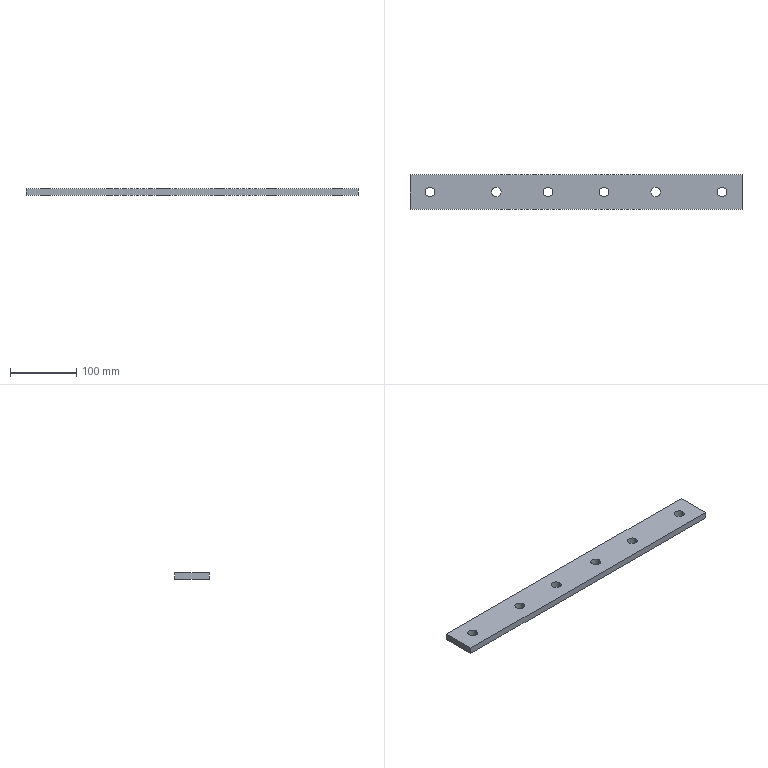Part | SolidWorks | features FlatPattern 1, ICE 1, MirrorPattern 1, SMBaseFlange 1, SheetMetal 1 | 1 solid | 18 faces | box 500 x 52 x 10 mm | volume 250092 mm3 | cylinder 12 | plane 6 | commonest cylinder face diameters 14.5 x12
STEP:
#1=CARTESIAN_POINT('',(-34.75,0.,-10.));
#2=VERTEX_POINT('',#1);
#3=CARTESIAN_POINT('',(-49.25,0.,-10.));
#4=VERTEX_POINT('',#3);
#5=CARTESIAN_POINT('',(-42.,0.,-10.));
#6=DIRECTION('',(0.,0.,-1.));
#7=DIRECTION('',(-1.,0.,0.));
#8=AXIS2_PLACEMENT_3D('',#5,#6,#7);
#9=CIRCLE('',#8,7.25);
#10=EDGE_CURVE('',#2,#4,#9,.T.);
#11=ORIENTED_EDGE('',*,*,#10,.T.);
#12=CARTESIAN_POINT('',(-49.25,0.,0.));
#13=VERTEX_POINT('',#12);
#14=CARTESIAN_POINT('',(-49.25,0.,-10.));
#15=DIRECTION('',(0.,0.,1.));
#16=VECTOR('',#15,1000.);
#17=LINE('',#14,#16);
#18=EDGE_CURVE('',#4,#13,#17,.T.);
#19=ORIENTED_EDGE('',*,*,#18,.T.);
#20=CARTESIAN_POINT('',(-34.75,0.,0.));
#21=VERTEX_POINT('',#20);
#22=CARTESIAN_POINT('',(-42.,0.,0.));
#23=DIRECTION('',(0.,0.,-1.));
#24=DIRECTION('',(1.,0.,0.));
#25=AXIS2_PLACEMENT_3D('',#22,#23,#24);
#26=CIRCLE('',#25,7.25);
#27=EDGE_CURVE('',#21,#13,#26,.T.);
#28=ORIENTED_EDGE('',*,*,#27,.F.);
#29=CARTESIAN_POINT('',(-34.75,0.,-10.));
#30=DIRECTION('',(0.,0.,1.));
#31=VECTOR('',#30,1000.);
#32=LINE('',#29,#31);
#33=EDGE_CURVE('',#2,#21,#32,.T.);
#34=ORIENTED_EDGE('',*,*,#33,.F.);
#35=EDGE_LOOP('',(#11,#19,#28,#34));
#36=FACE_OUTER_BOUND('',#35,.T.);
#37=CARTESIAN_POINT('',(-42.,0.,-10.));
#38=DIRECTION('',(0.,0.,1.));
#39=DIRECTION('',(1.,0.,0.));
#40=AXIS2_PLACEMENT_3D('',#37,#38,#39);
#41=CYLINDRICAL_SURFACE('',#40,7.25);
#42=ADVANCED_FACE('',(#36),#41,.F.);
#43=CARTESIAN_POINT('',(-112.75,0.,-10.));
#44=VERTEX_POINT('',#43);
#45=CARTESIAN_POINT('',(-127.25,0.,-10.));
#46=VERTEX_POINT('',#45);
#47=CARTESIAN_POINT('',(-120.,0.,-10.));
#48=DIRECTION('',(0.,0.,-1.));
#49=DIRECTION('',(-1.,0.,0.));
#50=AXIS2_PLACEMENT_3D('',#47,#48,#49);
#51=CIRCLE('',#50,7.25);
#52=EDGE_CURVE('',#44,#46,#51,.T.);
#53=ORIENTED_EDGE('',*,*,#52,.T.);
#54=CARTESIAN_POINT('',(-127.25,0.,0.));
#55=VERTEX_POINT('',#54);
#56=CARTESIAN_POINT('',(-127.25,0.,-10.));
#57=DIRECTION('',(0.,0.,1.));
#58=VECTOR('',#57,1000.);
#59=LINE('',#56,#58);
#60=EDGE_CURVE('',#46,#55,#59,.T.);
#61=ORIENTED_EDGE('',*,*,#60,.T.);
#62=CARTESIAN_POINT('',(-112.75,0.,0.));
#63=VERTEX_POINT('',#62);
#64=CARTESIAN_POINT('',(-120.,0.,0.));
#65=DIRECTION('',(0.,0.,-1.));
#66=DIRECTION('',(1.,0.,0.));
#67=AXIS2_PLACEMENT_3D('',#64,#65,#66);
#68=CIRCLE('',#67,7.25);
#69=EDGE_CURVE('',#63,#55,#68,.T.);
#70=ORIENTED_EDGE('',*,*,#69,.F.);
#71=CARTESIAN_POINT('',(-112.75,0.,-10.));
#72=DIRECTION('',(0.,0.,1.));
#73=VECTOR('',#72,1000.);
#74=LINE('',#71,#73);
#75=EDGE_CURVE('',#44,#63,#74,.T.);
#76=ORIENTED_EDGE('',*,*,#75,.F.);
#77=EDGE_LOOP('',(#53,#61,#70,#76));
#78=FACE_OUTER_BOUND('',#77,.T.);
#79=CARTESIAN_POINT('',(-120.,0.,-10.));
#80=DIRECTION('',(0.,0.,1.));
#81=DIRECTION('',(1.,0.,0.));
#82=AXIS2_PLACEMENT_3D('',#79,#80,#81);
#83=CYLINDRICAL_SURFACE('',#82,7.25);
#84=ADVANCED_FACE('',(#78),#83,.F.);
#85=CARTESIAN_POINT('',(-212.75,0.,-10.));
#86=VERTEX_POINT('',#85);
#87=CARTESIAN_POINT('',(-227.25,0.,-10.));
#88=VERTEX_POINT('',#87);
#89=CARTESIAN_POINT('',(-220.,0.,-10.));
#90=DIRECTION('',(0.,0.,-1.));
#91=DIRECTION('',(-1.,0.,0.));
#92=AXIS2_PLACEMENT_3D('',#89,#90,#91);
#93=CIRCLE('',#92,7.25);
#94=EDGE_CURVE('',#86,#88,#93,.T.);
#95=ORIENTED_EDGE('',*,*,#94,.T.);
#96=CARTESIAN_POINT('',(-227.25,0.,0.));
#97=VERTEX_POINT('',#96);
#98=CARTESIAN_POINT('',(-227.25,0.,-10.));
#99=DIRECTION('',(0.,0.,1.));
#100=VECTOR('',#99,1000.);
#101=LINE('',#98,#100);
#102=EDGE_CURVE('',#88,#97,#101,.T.);
#103=ORIENTED_EDGE('',*,*,#102,.T.);
#104=CARTESIAN_POINT('',(-212.75,0.,0.));
#105=VERTEX_POINT('',#104);
#106=CARTESIAN_POINT('',(-220.,0.,0.));
#107=DIRECTION('',(0.,0.,-1.));
#108=DIRECTION('',(1.,0.,0.));
#109=AXIS2_PLACEMENT_3D('',#106,#107,#108);
#110=CIRCLE('',#109,7.25);
#111=EDGE_CURVE('',#105,#97,#110,.T.);
#112=ORIENTED_EDGE('',*,*,#111,.F.);
#113=CARTESIAN_POINT('',(-212.75,0.,-10.));
#114=DIRECTION('',(0.,0.,1.));
#115=VECTOR('',#114,1000.);
#116=LINE('',#113,#115);
#117=EDGE_CURVE('',#86,#105,#116,.T.);
#118=ORIENTED_EDGE('',*,*,#117,.F.);
#119=EDGE_LOOP('',(#95,#103,#112,#118));
#120=FACE_OUTER_BOUND('',#119,.T.);
#121=CARTESIAN_POINT('',(-220.,0.,-10.));
#122=DIRECTION('',(0.,0.,1.));
#123=DIRECTION('',(1.,0.,0.));
#124=AXIS2_PLACEMENT_3D('',#121,#122,#123);
#125=CYLINDRICAL_SURFACE('',#124,7.25);
#126=ADVANCED_FACE('',(#120),#125,.F.);
#127=CARTESIAN_POINT('',(34.75,0.,-10.));
#128=VERTEX_POINT('',#127);
#129=CARTESIAN_POINT('',(49.25,0.,-10.));
#130=VERTEX_POINT('',#129);
#131=CARTESIAN_POINT('',(42.,0.,-10.));
#132=DIRECTION('',(0.,0.,1.));
#133=DIRECTION('',(1.,0.,0.));
#134=AXIS2_PLACEMENT_3D('',#131,#132,#133);
#135=CIRCLE('',#134,7.25);
#136=EDGE_CURVE('',#128,#130,#135,.T.);
#137=ORIENTED_EDGE('',*,*,#136,.F.);
#138=CARTESIAN_POINT('',(34.75,0.,0.));
#139=VERTEX_POINT('',#138);
#140=CARTESIAN_POINT('',(34.75,0.,-10.));
#141=DIRECTION('',(0.,0.,1.));
#142=VECTOR('',#141,1000.);
#143=LINE('',#140,#142);
#144=EDGE_CURVE('',#128,#139,#143,.T.);
#145=ORIENTED_EDGE('',*,*,#144,.T.);
#146=CARTESIAN_POINT('',(49.25,0.,0.));
#147=VERTEX_POINT('',#146);
#148=CARTESIAN_POINT('',(42.,0.,0.));
#149=DIRECTION('',(0.,0.,1.));
#150=DIRECTION('',(1.,0.,0.));
#151=AXIS2_PLACEMENT_3D('',#148,#149,#150);
#152=CIRCLE('',#151,7.25);
#153=EDGE_CURVE('',#139,#147,#152,.T.);
#154=ORIENTED_EDGE('',*,*,#153,.T.);
#155=CARTESIAN_POINT('',(49.25,0.,-10.));
#156=DIRECTION('',(0.,0.,1.));
#157=VECTOR('',#156,1000.);
#158=LINE('',#155,#157);
#159=EDGE_CURVE('',#130,#147,#158,.T.);
#160=ORIENTED_EDGE('',*,*,#159,.F.);
#161=EDGE_LOOP('',(#137,#145,#154,#160));
#162=FACE_OUTER_BOUND('',#161,.T.);
#163=CARTESIAN_POINT('',(42.,0.,-10.));
#164=DIRECTION('',(0.,0.,1.));
#165=DIRECTION('',(1.,0.,0.));
#166=AXIS2_PLACEMENT_3D('',#163,#164,#165);
#167=CYLINDRICAL_SURFACE('',#166,7.25);
#168=ADVANCED_FACE('',(#162),#167,.F.);
#169=CARTESIAN_POINT('',(112.75,0.,-10.));
#170=VERTEX_POINT('',#169);
#171=CARTESIAN_POINT('',(127.25,0.,-10.));
#172=VERTEX_POINT('',#171);
#173=CARTESIAN_POINT('',(120.,0.,-10.));
#174=DIRECTION('',(0.,0.,1.));
#175=DIRECTION('',(1.,0.,0.));
#176=AXIS2_PLACEMENT_3D('',#173,#174,#175);
#177=CIRCLE('',#176,7.25);
#178=EDGE_CURVE('',#170,#172,#177,.T.);
#179=ORIENTED_EDGE('',*,*,#178,.F.);
#180=CARTESIAN_POINT('',(112.75,0.,0.));
#181=VERTEX_POINT('',#180);
#182=CARTESIAN_POINT('',(112.75,0.,-10.));
#183=DIRECTION('',(0.,0.,1.));
#184=VECTOR('',#183,1000.);
#185=LINE('',#182,#184);
#186=EDGE_CURVE('',#170,#181,#185,.T.);
#187=ORIENTED_EDGE('',*,*,#186,.T.);
#188=CARTESIAN_POINT('',(127.25,0.,0.));
#189=VERTEX_POINT('',#188);
#190=CARTESIAN_POINT('',(120.,0.,0.));
#191=DIRECTION('',(0.,0.,1.));
#192=DIRECTION('',(1.,0.,0.));
#193=AXIS2_PLACEMENT_3D('',#190,#191,#192);
#194=CIRCLE('',#193,7.25);
#195=EDGE_CURVE('',#181,#189,#194,.T.);
#196=ORIENTED_EDGE('',*,*,#195,.T.);
#197=CARTESIAN_POINT('',(127.25,0.,-10.));
#198=DIRECTION('',(0.,0.,1.));
#199=VECTOR('',#198,1000.);
#200=LINE('',#197,#199);
#201=EDGE_CURVE('',#172,#189,#200,.T.);
#202=ORIENTED_EDGE('',*,*,#201,.F.);
#203=EDGE_LOOP('',(#179,#187,#196,#202));
#204=FACE_OUTER_BOUND('',#203,.T.);
#205=CARTESIAN_POINT('',(120.,0.,-10.));
#206=DIRECTION('',(0.,0.,1.));
#207=DIRECTION('',(1.,0.,0.));
#208=AXIS2_PLACEMENT_3D('',#205,#206,#207);
#209=CYLINDRICAL_SURFACE('',#208,7.25);
#210=ADVANCED_FACE('',(#204),#209,.F.);
#211=CARTESIAN_POINT('',(212.75,0.,-10.));
#212=VERTEX_POINT('',#211);
#213=CARTESIAN_POINT('',(227.25,0.,-10.));
#214=VERTEX_POINT('',#213);
#215=CARTESIAN_POINT('',(220.,0.,-10.));
#216=DIRECTION('',(0.,0.,1.));
#217=DIRECTION('',(1.,0.,0.));
#218=AXIS2_PLACEMENT_3D('',#215,#216,#217);
#219=CIRCLE('',#218,7.25);
#220=EDGE_CURVE('',#212,#214,#219,.T.);
#221=ORIENTED_EDGE('',*,*,#220,.F.);
#222=CARTESIAN_POINT('',(212.75,0.,0.));
#223=VERTEX_POINT('',#222);
#224=CARTESIAN_POINT('',(212.75,0.,-10.));
#225=DIRECTION('',(0.,0.,1.));
#226=VECTOR('',#225,1000.);
#227=LINE('',#224,#226);
#228=EDGE_CURVE('',#212,#223,#227,.T.);
#229=ORIENTED_EDGE('',*,*,#228,.T.);
#230=CARTESIAN_POINT('',(227.25,0.,0.));
#231=VERTEX_POINT('',#230);
#232=CARTESIAN_POINT('',(220.,0.,0.));
#233=DIRECTION('',(0.,0.,1.));
#234=DIRECTION('',(1.,0.,0.));
#235=AXIS2_PLACEMENT_3D('',#232,#233,#234);
#236=CIRCLE('',#235,7.25);
#237=EDGE_CURVE('',#223,#231,#236,.T.);
#238=ORIENTED_EDGE('',*,*,#237,.T.);
#239=CARTESIAN_POINT('',(227.25,0.,-10.));
#240=DIRECTION('',(0.,0.,1.));
#241=VECTOR('',#240,1000.);
#242=LINE('',#239,#241);
#243=EDGE_CURVE('',#214,#231,#242,.T.);
#244=ORIENTED_EDGE('',*,*,#243,.F.);
#245=EDGE_LOOP('',(#221,#229,#238,#244));
#246=FACE_OUTER_BOUND('',#245,.T.);
#247=CARTESIAN_POINT('',(220.,0.,-10.));
#248=DIRECTION('',(0.,0.,1.));
#249=DIRECTION('',(1.,0.,0.));
#250=AXIS2_PLACEMENT_3D('',#247,#248,#249);
#251=CYLINDRICAL_SURFACE('',#250,7.25);
#252=ADVANCED_FACE('',(#246),#251,.F.);
#253=CARTESIAN_POINT('',(250.,-26.,0.));
#254=VERTEX_POINT('',#253);
#255=CARTESIAN_POINT('',(250.,26.,0.));
#256=VERTEX_POINT('',#255);
#257=CARTESIAN_POINT('',(250.,26.,0.));
#258=DIRECTION('',(0.,1.,0.));
#259=VECTOR('',#258,1000.);
#260=LINE('',#257,#259);
#261=EDGE_CURVE('',#254,#256,#260,.T.);
#262=ORIENTED_EDGE('',*,*,#261,.F.);
#263=CARTESIAN_POINT('',(250.,-26.,-10.));
#264=VERTEX_POINT('',#263);
#265=CARTESIAN_POINT('',(250.,-26.,-10.));
#266=DIRECTION('',(0.,0.,1.));
#267=VECTOR('',#266,1000.);
#268=LINE('',#265,#267);
#269=EDGE_CURVE('',#264,#254,#268,.T.);
#270=ORIENTED_EDGE('',*,*,#269,.F.);
#271=CARTESIAN_POINT('',(250.,26.,-10.));
#272=VERTEX_POINT('',#271);
#273=CARTESIAN_POINT('',(250.,26.,-10.));
#274=DIRECTION('',(0.,1.,0.));
#275=VECTOR('',#274,1000.);
#276=LINE('',#273,#275);
#277=EDGE_CURVE('',#264,#272,#276,.T.);
#278=ORIENTED_EDGE('',*,*,#277,.T.);
#279=CARTESIAN_POINT('',(250.,26.,-10.));
#280=DIRECTION('',(0.,0.,1.));
#281=VECTOR('',#280,1000.);
#282=LINE('',#279,#281);
#283=EDGE_CURVE('',#272,#256,#282,.T.);
#284=ORIENTED_EDGE('',*,*,#283,.T.);
#285=EDGE_LOOP('',(#262,#270,#278,#284));
#286=FACE_OUTER_BOUND('',#285,.T.);
#287=CARTESIAN_POINT('',(250.,26.,-10.));
#288=DIRECTION('',(1.,0.,0.));
#289=DIRECTION('',(0.,0.,-1.));
#290=AXIS2_PLACEMENT_3D('',#287,#288,#289);
#291=PLANE('',#290);
#292=ADVANCED_FACE('',(#286),#291,.T.);
#293=CARTESIAN_POINT('',(-250.,-26.,0.));
#294=VERTEX_POINT('',#293);
#295=CARTESIAN_POINT('',(-250.,-26.,0.));
#296=DIRECTION('',(1.,0.,0.));
#297=VECTOR('',#296,1000.);
#298=LINE('',#295,#297);
#299=EDGE_CURVE('',#294,#254,#298,.T.);
#300=ORIENTED_EDGE('',*,*,#299,.F.);
#301=CARTESIAN_POINT('',(-250.,-26.,-10.));
#302=VERTEX_POINT('',#301);
#303=CARTESIAN_POINT('',(-250.,-26.,-10.));
#304=DIRECTION('',(0.,0.,1.));
#305=VECTOR('',#304,1000.);
#306=LINE('',#303,#305);
#307=EDGE_CURVE('',#302,#294,#306,.T.);
#308=ORIENTED_EDGE('',*,*,#307,.F.);
#309=CARTESIAN_POINT('',(-250.,-26.,-10.));
#310=DIRECTION('',(1.,0.,0.));
#311=VECTOR('',#310,1000.);
#312=LINE('',#309,#311);
#313=EDGE_CURVE('',#302,#264,#312,.T.);
#314=ORIENTED_EDGE('',*,*,#313,.T.);
#315=ORIENTED_EDGE('',*,*,#269,.T.);
#316=EDGE_LOOP('',(#300,#308,#314,#315));
#317=FACE_OUTER_BOUND('',#316,.T.);
#318=CARTESIAN_POINT('',(-250.,-26.,-10.));
#319=DIRECTION('',(0.,-1.,0.));
#320=DIRECTION('',(0.,0.,-1.));
#321=AXIS2_PLACEMENT_3D('',#318,#319,#320);
#322=PLANE('',#321);
#323=ADVANCED_FACE('',(#317),#322,.T.);
#324=CARTESIAN_POINT('',(-250.,26.,0.));
#325=VERTEX_POINT('',#324);
#326=CARTESIAN_POINT('',(-250.,26.,0.));
#327=DIRECTION('',(0.,-1.,0.));
#328=VECTOR('',#327,1000.);
#329=LINE('',#326,#328);
#330=EDGE_CURVE('',#325,#294,#329,.T.);
#331=ORIENTED_EDGE('',*,*,#330,.F.);
#332=CARTESIAN_POINT('',(-250.,26.,-10.));
#333=VERTEX_POINT('',#332);
#334=CARTESIAN_POINT('',(-250.,26.,-10.));
#335=DIRECTION('',(0.,0.,1.));
#336=VECTOR('',#335,1000.);
#337=LINE('',#334,#336);
#338=EDGE_CURVE('',#333,#325,#337,.T.);
#339=ORIENTED_EDGE('',*,*,#338,.F.);
#340=CARTESIAN_POINT('',(-250.,26.,-10.));
#341=DIRECTION('',(0.,-1.,0.));
#342=VECTOR('',#341,1000.);
#343=LINE('',#340,#342);
#344=EDGE_CURVE('',#333,#302,#343,.T.);
#345=ORIENTED_EDGE('',*,*,#344,.T.);
#346=ORIENTED_EDGE('',*,*,#307,.T.);
#347=EDGE_LOOP('',(#331,#339,#345,#346));
#348=FACE_OUTER_BOUND('',#347,.T.);
#349=CARTESIAN_POINT('',(-250.,26.,-10.));
#350=DIRECTION('',(-1.,0.,0.));
#351=DIRECTION('',(0.,0.,1.));
#352=AXIS2_PLACEMENT_3D('',#349,#350,#351);
#353=PLANE('',#352);
#354=ADVANCED_FACE('',(#348),#353,.T.);
#355=CARTESIAN_POINT('',(-250.,26.,0.));
#356=DIRECTION('',(-1.,0.,0.));
#357=VECTOR('',#356,1000.);
#358=LINE('',#355,#357);
#359=EDGE_CURVE('',#256,#325,#358,.T.);
#360=ORIENTED_EDGE('',*,*,#359,.F.);
#361=ORIENTED_EDGE('',*,*,#283,.F.);
#362=CARTESIAN_POINT('',(-250.,26.,-10.));
#363=DIRECTION('',(-1.,0.,0.));
#364=VECTOR('',#363,1000.);
#365=LINE('',#362,#364);
#366=EDGE_CURVE('',#272,#333,#365,.T.);
#367=ORIENTED_EDGE('',*,*,#366,.T.);
#368=ORIENTED_EDGE('',*,*,#338,.T.);
#369=EDGE_LOOP('',(#360,#361,#367,#368));
#370=FACE_OUTER_BOUND('',#369,.T.);
#371=CARTESIAN_POINT('',(-250.,26.,-10.));
#372=DIRECTION('',(0.,1.,0.));
#373=DIRECTION('',(0.,0.,1.));
#374=AXIS2_PLACEMENT_3D('',#371,#372,#373);
#375=PLANE('',#374);
#376=ADVANCED_FACE('',(#370),#375,.T.);
#377=ORIENTED_EDGE('',*,*,#10,.F.);
#378=CARTESIAN_POINT('',(-42.,0.,-10.));
#379=DIRECTION('',(0.,0.,-1.));
#380=DIRECTION('',(-1.,0.,0.));
#381=AXIS2_PLACEMENT_3D('',#378,#379,#380);
#382=CIRCLE('',#381,7.25);
#383=EDGE_CURVE('',#4,#2,#382,.T.);
#384=ORIENTED_EDGE('',*,*,#383,.F.);
#385=EDGE_LOOP('',(#377,#384));
#386=FACE_BOUND('',#385,.T.);
#387=ORIENTED_EDGE('',*,*,#52,.F.);
#388=CARTESIAN_POINT('',(-120.,0.,-10.));
#389=DIRECTION('',(0.,0.,-1.));
#390=DIRECTION('',(-1.,0.,0.));
#391=AXIS2_PLACEMENT_3D('',#388,#389,#390);
#392=CIRCLE('',#391,7.25);
#393=EDGE_CURVE('',#46,#44,#392,.T.);
#394=ORIENTED_EDGE('',*,*,#393,.F.);
#395=EDGE_LOOP('',(#387,#394));
#396=FACE_BOUND('',#395,.T.);
#397=ORIENTED_EDGE('',*,*,#94,.F.);
#398=CARTESIAN_POINT('',(-220.,0.,-10.));
#399=DIRECTION('',(0.,0.,-1.));
#400=DIRECTION('',(-1.,0.,0.));
#401=AXIS2_PLACEMENT_3D('',#398,#399,#400);
#402=CIRCLE('',#401,7.25);
#403=EDGE_CURVE('',#88,#86,#402,.T.);
#404=ORIENTED_EDGE('',*,*,#403,.F.);
#405=EDGE_LOOP('',(#397,#404));
#406=FACE_BOUND('',#405,.T.);
#407=CARTESIAN_POINT('',(42.,0.,-10.));
#408=DIRECTION('',(0.,0.,1.));
#409=DIRECTION('',(1.,0.,0.));
#410=AXIS2_PLACEMENT_3D('',#407,#408,#409);
#411=CIRCLE('',#410,7.25);
#412=EDGE_CURVE('',#130,#128,#411,.T.);
#413=ORIENTED_EDGE('',*,*,#412,.T.);
#414=ORIENTED_EDGE('',*,*,#136,.T.);
#415=EDGE_LOOP('',(#413,#414));
#416=FACE_BOUND('',#415,.T.);
#417=CARTESIAN_POINT('',(120.,0.,-10.));
#418=DIRECTION('',(0.,0.,1.));
#419=DIRECTION('',(1.,0.,0.));
#420=AXIS2_PLACEMENT_3D('',#417,#418,#419);
#421=CIRCLE('',#420,7.25);
#422=EDGE_CURVE('',#172,#170,#421,.T.);
#423=ORIENTED_EDGE('',*,*,#422,.T.);
#424=ORIENTED_EDGE('',*,*,#178,.T.);
#425=EDGE_LOOP('',(#423,#424));
#426=FACE_BOUND('',#425,.T.);
#427=CARTESIAN_POINT('',(220.,0.,-10.));
#428=DIRECTION('',(0.,0.,1.));
#429=DIRECTION('',(1.,0.,0.));
#430=AXIS2_PLACEMENT_3D('',#427,#428,#429);
#431=CIRCLE('',#430,7.25);
#432=EDGE_CURVE('',#214,#212,#431,.T.);
#433=ORIENTED_EDGE('',*,*,#432,.T.);
#434=ORIENTED_EDGE('',*,*,#220,.T.);
#435=EDGE_LOOP('',(#433,#434));
#436=FACE_BOUND('',#435,.T.);
#437=ORIENTED_EDGE('',*,*,#277,.F.);
#438=ORIENTED_EDGE('',*,*,#313,.F.);
#439=ORIENTED_EDGE('',*,*,#344,.F.);
#440=ORIENTED_EDGE('',*,*,#366,.F.);
#441=EDGE_LOOP('',(#437,#438,#439,#440));
#442=FACE_OUTER_BOUND('',#441,.T.);
#443=CARTESIAN_POINT('',(0.,0.,-10.));
#444=DIRECTION('',(0.,0.,1.));
#445=DIRECTION('',(1.,0.,0.));
#446=AXIS2_PLACEMENT_3D('',#443,#444,#445);
#447=PLANE('',#446);
#448=ADVANCED_FACE('',(#386,#396,#406,#416,#426,#436,#442),#447,.F.);
#449=ORIENTED_EDGE('',*,*,#27,.T.);
#450=CARTESIAN_POINT('',(-42.,0.,0.));
#451=DIRECTION('',(0.,0.,-1.));
#452=DIRECTION('',(1.,0.,0.));
#453=AXIS2_PLACEMENT_3D('',#450,#451,#452);
#454=CIRCLE('',#453,7.25);
#455=EDGE_CURVE('',#13,#21,#454,.T.);
#456=ORIENTED_EDGE('',*,*,#455,.T.);
#457=EDGE_LOOP('',(#449,#456));
#458=FACE_BOUND('',#457,.T.);
#459=ORIENTED_EDGE('',*,*,#69,.T.);
#460=CARTESIAN_POINT('',(-120.,0.,0.));
#461=DIRECTION('',(0.,0.,-1.));
#462=DIRECTION('',(1.,0.,0.));
#463=AXIS2_PLACEMENT_3D('',#460,#461,#462);
#464=CIRCLE('',#463,7.25);
#465=EDGE_CURVE('',#55,#63,#464,.T.);
#466=ORIENTED_EDGE('',*,*,#465,.T.);
#467=EDGE_LOOP('',(#459,#466));
#468=FACE_BOUND('',#467,.T.);
#469=ORIENTED_EDGE('',*,*,#111,.T.);
#470=CARTESIAN_POINT('',(-220.,0.,0.));
#471=DIRECTION('',(0.,0.,-1.));
#472=DIRECTION('',(1.,0.,0.));
#473=AXIS2_PLACEMENT_3D('',#470,#471,#472);
#474=CIRCLE('',#473,7.25);
#475=EDGE_CURVE('',#97,#105,#474,.T.);
#476=ORIENTED_EDGE('',*,*,#475,.T.);
#477=EDGE_LOOP('',(#469,#476));
#478=FACE_BOUND('',#477,.T.);
#479=CARTESIAN_POINT('',(42.,0.,0.));
#480=DIRECTION('',(0.,0.,1.));
#481=DIRECTION('',(1.,0.,0.));
#482=AXIS2_PLACEMENT_3D('',#479,#480,#481);
#483=CIRCLE('',#482,7.25);
#484=EDGE_CURVE('',#147,#139,#483,.T.);
#485=ORIENTED_EDGE('',*,*,#484,.F.);
#486=ORIENTED_EDGE('',*,*,#153,.F.);
#487=EDGE_LOOP('',(#485,#486));
#488=FACE_BOUND('',#487,.T.);
#489=CARTESIAN_POINT('',(120.,0.,0.));
#490=DIRECTION('',(0.,0.,1.));
#491=DIRECTION('',(1.,0.,0.));
#492=AXIS2_PLACEMENT_3D('',#489,#490,#491);
#493=CIRCLE('',#492,7.25);
#494=EDGE_CURVE('',#189,#181,#493,.T.);
#495=ORIENTED_EDGE('',*,*,#494,.F.);
#496=ORIENTED_EDGE('',*,*,#195,.F.);
#497=EDGE_LOOP('',(#495,#496));
#498=FACE_BOUND('',#497,.T.);
#499=CARTESIAN_POINT('',(220.,0.,0.));
#500=DIRECTION('',(0.,0.,1.));
#501=DIRECTION('',(1.,0.,0.));
#502=AXIS2_PLACEMENT_3D('',#499,#500,#501);
#503=CIRCLE('',#502,7.25);
#504=EDGE_CURVE('',#231,#223,#503,.T.);
#505=ORIENTED_EDGE('',*,*,#504,.F.);
#506=ORIENTED_EDGE('',*,*,#237,.F.);
#507=EDGE_LOOP('',(#505,#506));
#508=FACE_BOUND('',#507,.T.);
#509=ORIENTED_EDGE('',*,*,#261,.T.);
#510=ORIENTED_EDGE('',*,*,#359,.T.);
#511=ORIENTED_EDGE('',*,*,#330,.T.);
#512=ORIENTED_EDGE('',*,*,#299,.T.);
#513=EDGE_LOOP('',(#509,#510,#511,#512));
#514=FACE_OUTER_BOUND('',#513,.T.);
#515=CARTESIAN_POINT('',(0.,0.,0.));
#516=DIRECTION('',(0.,0.,1.));
#517=DIRECTION('',(1.,0.,0.));
#518=AXIS2_PLACEMENT_3D('',#515,#516,#517);
#519=PLANE('',#518);
#520=ADVANCED_FACE('',(#458,#468,#478,#488,#498,#508,#514),#519,.T.);
#521=ORIENTED_EDGE('',*,*,#228,.F.);
#522=ORIENTED_EDGE('',*,*,#432,.F.);
#523=ORIENTED_EDGE('',*,*,#243,.T.);
#524=ORIENTED_EDGE('',*,*,#504,.T.);
#525=EDGE_LOOP('',(#521,#522,#523,#524));
#526=FACE_OUTER_BOUND('',#525,.T.);
#527=CARTESIAN_POINT('',(220.,0.,-10.));
#528=DIRECTION('',(0.,0.,1.));
#529=DIRECTION('',(1.,0.,0.));
#530=AXIS2_PLACEMENT_3D('',#527,#528,#529);
#531=CYLINDRICAL_SURFACE('',#530,7.25);
#532=ADVANCED_FACE('',(#526),#531,.F.);
#533=ORIENTED_EDGE('',*,*,#186,.F.);
#534=ORIENTED_EDGE('',*,*,#422,.F.);
#535=ORIENTED_EDGE('',*,*,#201,.T.);
#536=ORIENTED_EDGE('',*,*,#494,.T.);
#537=EDGE_LOOP('',(#533,#534,#535,#536));
#538=FACE_OUTER_BOUND('',#537,.T.);
#539=CARTESIAN_POINT('',(120.,0.,-10.));
#540=DIRECTION('',(0.,0.,1.));
#541=DIRECTION('',(1.,0.,0.));
#542=AXIS2_PLACEMENT_3D('',#539,#540,#541);
#543=CYLINDRICAL_SURFACE('',#542,7.25);
#544=ADVANCED_FACE('',(#538),#543,.F.);
#545=ORIENTED_EDGE('',*,*,#144,.F.);
#546=ORIENTED_EDGE('',*,*,#412,.F.);
#547=ORIENTED_EDGE('',*,*,#159,.T.);
#548=ORIENTED_EDGE('',*,*,#484,.T.);
#549=EDGE_LOOP('',(#545,#546,#547,#548));
#550=FACE_OUTER_BOUND('',#549,.T.);
#551=CARTESIAN_POINT('',(42.,0.,-10.));
#552=DIRECTION('',(0.,0.,1.));
#553=DIRECTION('',(1.,0.,0.));
#554=AXIS2_PLACEMENT_3D('',#551,#552,#553);
#555=CYLINDRICAL_SURFACE('',#554,7.25);
#556=ADVANCED_FACE('',(#550),#555,.F.);
#557=ORIENTED_EDGE('',*,*,#102,.F.);
#558=ORIENTED_EDGE('',*,*,#403,.T.);
#559=ORIENTED_EDGE('',*,*,#117,.T.);
#560=ORIENTED_EDGE('',*,*,#475,.F.);
#561=EDGE_LOOP('',(#557,#558,#559,#560));
#562=FACE_OUTER_BOUND('',#561,.T.);
#563=CARTESIAN_POINT('',(-220.,0.,-10.));
#564=DIRECTION('',(0.,0.,1.));
#565=DIRECTION('',(1.,0.,0.));
#566=AXIS2_PLACEMENT_3D('',#563,#564,#565);
#567=CYLINDRICAL_SURFACE('',#566,7.25);
#568=ADVANCED_FACE('',(#562),#567,.F.);
#569=ORIENTED_EDGE('',*,*,#60,.F.);
#570=ORIENTED_EDGE('',*,*,#393,.T.);
#571=ORIENTED_EDGE('',*,*,#75,.T.);
#572=ORIENTED_EDGE('',*,*,#465,.F.);
#573=EDGE_LOOP('',(#569,#570,#571,#572));
#574=FACE_OUTER_BOUND('',#573,.T.);
#575=CARTESIAN_POINT('',(-120.,0.,-10.));
#576=DIRECTION('',(0.,0.,1.));
#577=DIRECTION('',(1.,0.,0.));
#578=AXIS2_PLACEMENT_3D('',#575,#576,#577);
#579=CYLINDRICAL_SURFACE('',#578,7.25);
#580=ADVANCED_FACE('',(#574),#579,.F.);
#581=ORIENTED_EDGE('',*,*,#18,.F.);
#582=ORIENTED_EDGE('',*,*,#383,.T.);
#583=ORIENTED_EDGE('',*,*,#33,.T.);
#584=ORIENTED_EDGE('',*,*,#455,.F.);
#585=EDGE_LOOP('',(#581,#582,#583,#584));
#586=FACE_OUTER_BOUND('',#585,.T.);
#587=CARTESIAN_POINT('',(-42.,0.,-10.));
#588=DIRECTION('',(0.,0.,1.));
#589=DIRECTION('',(1.,0.,0.));
#590=AXIS2_PLACEMENT_3D('',#587,#588,#589);
#591=CYLINDRICAL_SURFACE('',#590,7.25);
#592=ADVANCED_FACE('',(#586),#591,.F.);
#593=CLOSED_SHELL('',(#42,#84,#126,#168,#210,#252,#292,#323,#354,#376,#448,#520,#532,#544,#556,#568,#580,#592));
#594=MANIFOLD_SOLID_BREP('',#593);
#595=CARTESIAN_POINT('',(0.,0.,0.));
#596=DIRECTION('',(0.,0.,1.));
#597=DIRECTION('',(1.,0.,0.));
#598=AXIS2_PLACEMENT_3D('',#595,#596,#597);
#599=(LENGTH_UNIT()NAMED_UNIT(*)SI_UNIT(.MILLI.,.METRE.));
#600=UNCERTAINTY_MEASURE_WITH_UNIT(LENGTH_MEASURE(0.00001),#599,'','');
#601=(NAMED_UNIT(*)PLANE_ANGLE_UNIT()SI_UNIT($,.RADIAN.));
#602=(NAMED_UNIT(*)SI_UNIT($,.STERADIAN.)SOLID_ANGLE_UNIT());
#603=(GEOMETRIC_REPRESENTATION_CONTEXT(3)GLOBAL_UNCERTAINTY_ASSIGNED_CONTEXT((#600))GLOBAL_UNIT_ASSIGNED_CONTEXT((#599,#601,#602))REPRESENTATION_CONTEXT('',''));
#604=ADVANCED_BREP_SHAPE_REPRESENTATION('',(#594,#598),#603);